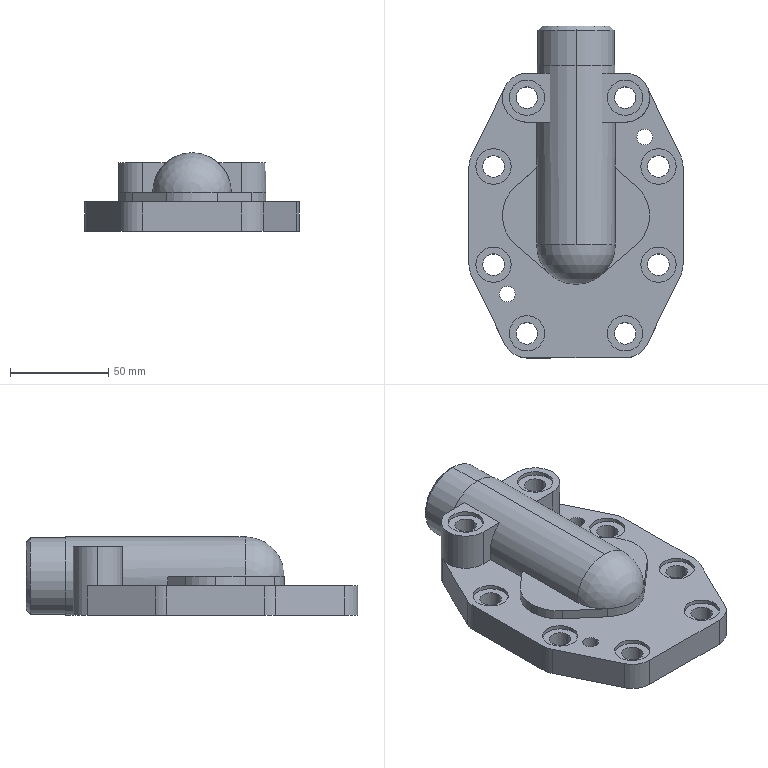Part | SolidWorks | features ICE 13, 3DProfileFeature 1, Dome 1, HoleWzd 1, MirrorPattern 1, StudWizard 1 | 1 solid | 126 faces | box 109 x 169 x 40 mm | volume 262615 mm3 | cylinder 67 | plane 51 | cone 7 | sphere 1 | commonest cylinder face diameters 11 x16 18 x16 25 x9 14 x8 40 x6 8 x4